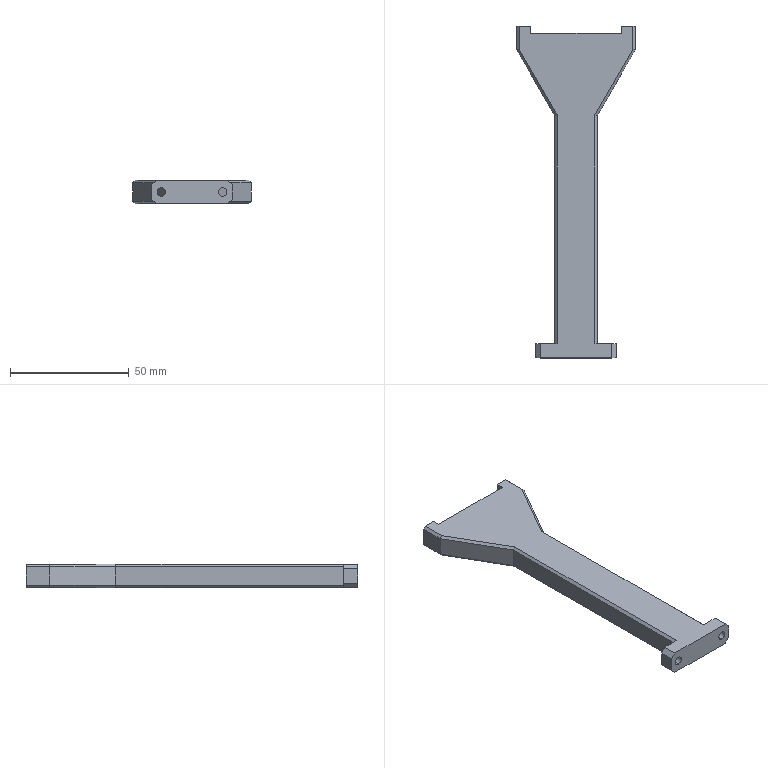Part | SolidWorks | features Chamfer 2, HoleWzd 2, ICE 2, Extrusion 1, MirrorPattern 1 | 1 solid | 46 faces | box 50 x 140 x 10 mm | volume 32128 mm3 | plane 34 | cylinder 8 | cone 4 | commonest cylinder face diameters 2.5 x4 3.5 x4
STEP:
#1=CARTESIAN_POINT('',(-13.,-64.,1.75));
#2=VERTEX_POINT('',#1);
#3=CARTESIAN_POINT('',(-13.,-64.,-1.75));
#4=VERTEX_POINT('',#3);
#5=CARTESIAN_POINT('',(-13.,-64.,0.));
#6=DIRECTION('',(0.,-1.,0.));
#7=DIRECTION('',(0.,0.,-1.));
#8=AXIS2_PLACEMENT_3D('',#5,#6,#7);
#9=CIRCLE('',#8,1.75);
#10=EDGE_CURVE('',#2,#4,#9,.T.);
#11=ORIENTED_EDGE('',*,*,#10,.F.);
#12=CARTESIAN_POINT('',(-13.,-70.,1.75));
#13=VERTEX_POINT('',#12);
#14=CARTESIAN_POINT('',(-13.,-70.,1.75));
#15=DIRECTION('',(0.,-1.,0.));
#16=VECTOR('',#15,1000.);
#17=LINE('',#14,#16);
#18=EDGE_CURVE('',#2,#13,#17,.T.);
#19=ORIENTED_EDGE('',*,*,#18,.T.);
#20=CARTESIAN_POINT('',(-13.,-70.,-1.75));
#21=VERTEX_POINT('',#20);
#22=CARTESIAN_POINT('',(-13.,-70.,0.));
#23=DIRECTION('',(0.,-1.,0.));
#24=DIRECTION('',(0.,0.,-1.));
#25=AXIS2_PLACEMENT_3D('',#22,#23,#24);
#26=CIRCLE('',#25,1.75);
#27=EDGE_CURVE('',#13,#21,#26,.T.);
#28=ORIENTED_EDGE('',*,*,#27,.T.);
#29=CARTESIAN_POINT('',(-13.,-70.,-1.75));
#30=DIRECTION('',(0.,-1.,0.));
#31=VECTOR('',#30,1000.);
#32=LINE('',#29,#31);
#33=EDGE_CURVE('',#4,#21,#32,.T.);
#34=ORIENTED_EDGE('',*,*,#33,.F.);
#35=EDGE_LOOP('',(#11,#19,#28,#34));
#36=FACE_OUTER_BOUND('',#35,.T.);
#37=CARTESIAN_POINT('',(-13.,-70.,0.));
#38=DIRECTION('',(0.,-1.,0.));
#39=DIRECTION('',(0.,0.,-1.));
#40=AXIS2_PLACEMENT_3D('',#37,#38,#39);
#41=CYLINDRICAL_SURFACE('',#40,1.75);
#42=ADVANCED_FACE('',(#36),#41,.F.);
#43=CARTESIAN_POINT('',(13.,-64.,-1.75));
#44=VERTEX_POINT('',#43);
#45=CARTESIAN_POINT('',(13.,-64.,1.75));
#46=VERTEX_POINT('',#45);
#47=CARTESIAN_POINT('',(13.,-64.,0.));
#48=DIRECTION('',(0.,1.,0.));
#49=DIRECTION('',(0.,0.,1.));
#50=AXIS2_PLACEMENT_3D('',#47,#48,#49);
#51=CIRCLE('',#50,1.75);
#52=EDGE_CURVE('',#44,#46,#51,.T.);
#53=ORIENTED_EDGE('',*,*,#52,.T.);
#54=CARTESIAN_POINT('',(13.,-70.,1.75));
#55=VERTEX_POINT('',#54);
#56=CARTESIAN_POINT('',(13.,-70.,1.75));
#57=DIRECTION('',(0.,-1.,0.));
#58=VECTOR('',#57,1000.);
#59=LINE('',#56,#58);
#60=EDGE_CURVE('',#46,#55,#59,.T.);
#61=ORIENTED_EDGE('',*,*,#60,.T.);
#62=CARTESIAN_POINT('',(13.,-70.,-1.75));
#63=VERTEX_POINT('',#62);
#64=CARTESIAN_POINT('',(13.,-70.,0.));
#65=DIRECTION('',(0.,-1.,0.));
#66=DIRECTION('',(0.,0.,-1.));
#67=AXIS2_PLACEMENT_3D('',#64,#65,#66);
#68=CIRCLE('',#67,1.75);
#69=EDGE_CURVE('',#55,#63,#68,.T.);
#70=ORIENTED_EDGE('',*,*,#69,.T.);
#71=CARTESIAN_POINT('',(13.,-70.,-1.75));
#72=DIRECTION('',(0.,-1.,0.));
#73=VECTOR('',#72,1000.);
#74=LINE('',#71,#73);
#75=EDGE_CURVE('',#44,#63,#74,.T.);
#76=ORIENTED_EDGE('',*,*,#75,.F.);
#77=EDGE_LOOP('',(#53,#61,#70,#76));
#78=FACE_OUTER_BOUND('',#77,.T.);
#79=CARTESIAN_POINT('',(13.,-70.,0.));
#80=DIRECTION('',(0.,-1.,0.));
#81=DIRECTION('',(0.,0.,-1.));
#82=AXIS2_PLACEMENT_3D('',#79,#80,#81);
#83=CYLINDRICAL_SURFACE('',#82,1.75);
#84=ADVANCED_FACE('',(#78),#83,.F.);
#85=CARTESIAN_POINT('',(-22.,61.5,-1.25));
#86=VERTEX_POINT('',#85);
#87=CARTESIAN_POINT('',(-22.,61.5,1.25));
#88=VERTEX_POINT('',#87);
#89=CARTESIAN_POINT('',(-22.,61.5,0.));
#90=DIRECTION('',(0.,1.,0.));
#91=DIRECTION('',(0.,0.,1.));
#92=AXIS2_PLACEMENT_3D('',#89,#90,#91);
#93=CIRCLE('',#92,1.25);
#94=EDGE_CURVE('',#86,#88,#93,.T.);
#95=ORIENTED_EDGE('',*,*,#94,.F.);
#96=CARTESIAN_POINT('',(-22.,70.,-1.25));
#97=VERTEX_POINT('',#96);
#98=CARTESIAN_POINT('',(-22.,70.,-1.25));
#99=DIRECTION('',(0.,1.,0.));
#100=VECTOR('',#99,1000.);
#101=LINE('',#98,#100);
#102=EDGE_CURVE('',#86,#97,#101,.T.);
#103=ORIENTED_EDGE('',*,*,#102,.T.);
#104=CARTESIAN_POINT('',(-22.,70.,1.25));
#105=VERTEX_POINT('',#104);
#106=CARTESIAN_POINT('',(-22.,70.,0.));
#107=DIRECTION('',(0.,1.,0.));
#108=DIRECTION('',(0.,0.,1.));
#109=AXIS2_PLACEMENT_3D('',#106,#107,#108);
#110=CIRCLE('',#109,1.25);
#111=EDGE_CURVE('',#97,#105,#110,.T.);
#112=ORIENTED_EDGE('',*,*,#111,.T.);
#113=CARTESIAN_POINT('',(-22.,70.,1.25));
#114=DIRECTION('',(0.,1.,0.));
#115=VECTOR('',#114,1000.);
#116=LINE('',#113,#115);
#117=EDGE_CURVE('',#88,#105,#116,.T.);
#118=ORIENTED_EDGE('',*,*,#117,.F.);
#119=EDGE_LOOP('',(#95,#103,#112,#118));
#120=FACE_OUTER_BOUND('',#119,.T.);
#121=CARTESIAN_POINT('',(-22.,70.,0.));
#122=DIRECTION('',(0.,1.,0.));
#123=DIRECTION('',(0.,0.,1.));
#124=AXIS2_PLACEMENT_3D('',#121,#122,#123);
#125=CYLINDRICAL_SURFACE('',#124,1.25);
#126=ADVANCED_FACE('',(#120),#125,.F.);
#127=CARTESIAN_POINT('',(-22.,60.749,0.));
#128=VERTEX_POINT('',#127);
#129=CARTESIAN_POINT('',(-22.,61.5,1.25));
#130=DIRECTION('',(0.,0.515,0.8572));
#131=VECTOR('',#130,1000.);
#132=LINE('',#129,#131);
#133=EDGE_CURVE('',#128,#88,#132,.T.);
#134=ORIENTED_EDGE('',*,*,#133,.F.);
#135=CARTESIAN_POINT('',(-22.,61.5,-1.25));
#136=DIRECTION('',(0.,0.515,-0.8572));
#137=VECTOR('',#136,1000.);
#138=LINE('',#135,#137);
#139=EDGE_CURVE('',#128,#86,#138,.T.);
#140=ORIENTED_EDGE('',*,*,#139,.T.);
#141=ORIENTED_EDGE('',*,*,#94,.T.);
#142=EDGE_LOOP('',(#134,#140,#141));
#143=FACE_OUTER_BOUND('',#142,.T.);
#144=CARTESIAN_POINT('',(-22.,61.5,0.));
#145=DIRECTION('',(0.,1.,0.));
#146=DIRECTION('',(0.,0.,1.));
#147=AXIS2_PLACEMENT_3D('',#144,#145,#146);
#148=CONICAL_SURFACE('',#147,1.25,1.03);
#149=ADVANCED_FACE('',(#143),#148,.F.);
#150=CARTESIAN_POINT('',(22.,61.5,-1.25));
#151=VERTEX_POINT('',#150);
#152=CARTESIAN_POINT('',(22.,61.5,1.25));
#153=VERTEX_POINT('',#152);
#154=CARTESIAN_POINT('',(22.,61.5,0.));
#155=DIRECTION('',(0.,1.,0.));
#156=DIRECTION('',(0.,0.,1.));
#157=AXIS2_PLACEMENT_3D('',#154,#155,#156);
#158=CIRCLE('',#157,1.25);
#159=EDGE_CURVE('',#151,#153,#158,.T.);
#160=ORIENTED_EDGE('',*,*,#159,.F.);
#161=CARTESIAN_POINT('',(22.,70.,-1.25));
#162=VERTEX_POINT('',#161);
#163=CARTESIAN_POINT('',(22.,70.,-1.25));
#164=DIRECTION('',(0.,1.,0.));
#165=VECTOR('',#164,1000.);
#166=LINE('',#163,#165);
#167=EDGE_CURVE('',#151,#162,#166,.T.);
#168=ORIENTED_EDGE('',*,*,#167,.T.);
#169=CARTESIAN_POINT('',(22.,70.,1.25));
#170=VERTEX_POINT('',#169);
#171=CARTESIAN_POINT('',(22.,70.,0.));
#172=DIRECTION('',(0.,1.,0.));
#173=DIRECTION('',(0.,0.,1.));
#174=AXIS2_PLACEMENT_3D('',#171,#172,#173);
#175=CIRCLE('',#174,1.25);
#176=EDGE_CURVE('',#162,#170,#175,.T.);
#177=ORIENTED_EDGE('',*,*,#176,.T.);
#178=CARTESIAN_POINT('',(22.,70.,1.25));
#179=DIRECTION('',(0.,1.,0.));
#180=VECTOR('',#179,1000.);
#181=LINE('',#178,#180);
#182=EDGE_CURVE('',#153,#170,#181,.T.);
#183=ORIENTED_EDGE('',*,*,#182,.F.);
#184=EDGE_LOOP('',(#160,#168,#177,#183));
#185=FACE_OUTER_BOUND('',#184,.T.);
#186=CARTESIAN_POINT('',(22.,70.,0.));
#187=DIRECTION('',(0.,1.,0.));
#188=DIRECTION('',(0.,0.,1.));
#189=AXIS2_PLACEMENT_3D('',#186,#187,#188);
#190=CYLINDRICAL_SURFACE('',#189,1.25);
#191=ADVANCED_FACE('',(#185),#190,.F.);
#192=CARTESIAN_POINT('',(22.,60.749,0.));
#193=VERTEX_POINT('',#192);
#194=CARTESIAN_POINT('',(22.,61.5,1.25));
#195=DIRECTION('',(0.,0.515,0.8572));
#196=VECTOR('',#195,1000.);
#197=LINE('',#194,#196);
#198=EDGE_CURVE('',#193,#153,#197,.T.);
#199=ORIENTED_EDGE('',*,*,#198,.F.);
#200=CARTESIAN_POINT('',(22.,61.5,-1.25));
#201=DIRECTION('',(0.,0.515,-0.8572));
#202=VECTOR('',#201,1000.);
#203=LINE('',#200,#202);
#204=EDGE_CURVE('',#193,#151,#203,.T.);
#205=ORIENTED_EDGE('',*,*,#204,.T.);
#206=ORIENTED_EDGE('',*,*,#159,.T.);
#207=EDGE_LOOP('',(#199,#205,#206));
#208=FACE_OUTER_BOUND('',#207,.T.);
#209=CARTESIAN_POINT('',(22.,61.5,0.));
#210=DIRECTION('',(0.,1.,0.));
#211=DIRECTION('',(0.,0.,1.));
#212=AXIS2_PLACEMENT_3D('',#209,#210,#211);
#213=CONICAL_SURFACE('',#212,1.25,1.03);
#214=ADVANCED_FACE('',(#208),#213,.F.);
#215=CARTESIAN_POINT('',(22.,70.,0.));
#216=DIRECTION('',(0.,1.,0.));
#217=DIRECTION('',(0.,0.,1.));
#218=AXIS2_PLACEMENT_3D('',#215,#216,#217);
#219=CIRCLE('',#218,1.25);
#220=EDGE_CURVE('',#170,#162,#219,.T.);
#221=ORIENTED_EDGE('',*,*,#220,.F.);
#222=ORIENTED_EDGE('',*,*,#176,.F.);
#223=EDGE_LOOP('',(#221,#222));
#224=FACE_BOUND('',#223,.T.);
#225=CARTESIAN_POINT('',(25.,70.,4.));
#226=VERTEX_POINT('',#225);
#227=CARTESIAN_POINT('',(25.,70.,-4.));
#228=VERTEX_POINT('',#227);
#229=CARTESIAN_POINT('',(25.,70.,5.));
#230=DIRECTION('',(0.,0.,-1.));
#231=VECTOR('',#230,1000.);
#232=LINE('',#229,#231);
#233=EDGE_CURVE('',#226,#228,#232,.T.);
#234=ORIENTED_EDGE('',*,*,#233,.T.);
#235=CARTESIAN_POINT('',(24.,70.,-5.));
#236=VERTEX_POINT('',#235);
#237=CARTESIAN_POINT('',(25.,70.,-4.));
#238=DIRECTION('',(-0.7071,0.,-0.7071));
#239=VECTOR('',#238,1000.);
#240=LINE('',#237,#239);
#241=EDGE_CURVE('',#228,#236,#240,.T.);
#242=ORIENTED_EDGE('',*,*,#241,.T.);
#243=CARTESIAN_POINT('',(19.,70.,-5.));
#244=VERTEX_POINT('',#243);
#245=CARTESIAN_POINT('',(-25.,70.,-5.));
#246=DIRECTION('',(-1.,0.,0.));
#247=VECTOR('',#246,1000.);
#248=LINE('',#245,#247);
#249=EDGE_CURVE('',#236,#244,#248,.T.);
#250=ORIENTED_EDGE('',*,*,#249,.T.);
#251=CARTESIAN_POINT('',(19.,70.,5.));
#252=VERTEX_POINT('',#251);
#253=CARTESIAN_POINT('',(19.,70.,-5.));
#254=DIRECTION('',(0.,0.,1.));
#255=VECTOR('',#254,1000.);
#256=LINE('',#253,#255);
#257=EDGE_CURVE('',#244,#252,#256,.T.);
#258=ORIENTED_EDGE('',*,*,#257,.T.);
#259=CARTESIAN_POINT('',(24.,70.,5.));
#260=VERTEX_POINT('',#259);
#261=CARTESIAN_POINT('',(-25.,70.,5.));
#262=DIRECTION('',(-1.,0.,0.));
#263=VECTOR('',#262,1000.);
#264=LINE('',#261,#263);
#265=EDGE_CURVE('',#260,#252,#264,.T.);
#266=ORIENTED_EDGE('',*,*,#265,.F.);
#267=CARTESIAN_POINT('',(24.,70.,5.));
#268=DIRECTION('',(0.7071,0.,-0.7071));
#269=VECTOR('',#268,1000.);
#270=LINE('',#267,#269);
#271=EDGE_CURVE('',#260,#226,#270,.T.);
#272=ORIENTED_EDGE('',*,*,#271,.T.);
#273=EDGE_LOOP('',(#234,#242,#250,#258,#266,#272));
#274=FACE_OUTER_BOUND('',#273,.T.);
#275=CARTESIAN_POINT('',(-25.,70.,5.));
#276=DIRECTION('',(0.,-1.,0.));
#277=DIRECTION('',(0.,0.,-1.));
#278=AXIS2_PLACEMENT_3D('',#275,#276,#277);
#279=PLANE('',#278);
#280=ADVANCED_FACE('',(#224,#274),#279,.F.);
#281=CARTESIAN_POINT('',(25.,60.,-4.));
#282=VERTEX_POINT('',#281);
#283=CARTESIAN_POINT('',(25.,60.,4.));
#284=VERTEX_POINT('',#283);
#285=CARTESIAN_POINT('',(25.,60.,-5.));
#286=DIRECTION('',(0.,0.,1.));
#287=VECTOR('',#286,1000.);
#288=LINE('',#285,#287);
#289=EDGE_CURVE('',#282,#284,#288,.T.);
#290=ORIENTED_EDGE('',*,*,#289,.F.);
#291=CARTESIAN_POINT('',(25.,70.,-4.));
#292=DIRECTION('',(0.,1.,0.));
#293=VECTOR('',#292,1000.);
#294=LINE('',#291,#293);
#295=EDGE_CURVE('',#282,#228,#294,.T.);
#296=ORIENTED_EDGE('',*,*,#295,.T.);
#297=ORIENTED_EDGE('',*,*,#233,.F.);
#298=CARTESIAN_POINT('',(25.,60.,4.));
#299=DIRECTION('',(0.,-1.,0.));
#300=VECTOR('',#299,1000.);
#301=LINE('',#298,#300);
#302=EDGE_CURVE('',#226,#284,#301,.T.);
#303=ORIENTED_EDGE('',*,*,#302,.T.);
#304=EDGE_LOOP('',(#290,#296,#297,#303));
#305=FACE_OUTER_BOUND('',#304,.T.);
#306=CARTESIAN_POINT('',(25.,70.,5.));
#307=DIRECTION('',(-1.,0.,0.));
#308=DIRECTION('',(0.,-1.,0.));
#309=AXIS2_PLACEMENT_3D('',#306,#307,#308);
#310=PLANE('',#309);
#311=ADVANCED_FACE('',(#305),#310,.F.);
#312=CARTESIAN_POINT('',(-13.,-70.,0.));
#313=DIRECTION('',(0.,-1.,0.));
#314=DIRECTION('',(0.,0.,-1.));
#315=AXIS2_PLACEMENT_3D('',#312,#313,#314);
#316=CIRCLE('',#315,1.75);
#317=EDGE_CURVE('',#21,#13,#316,.T.);
#318=ORIENTED_EDGE('',*,*,#317,.F.);
#319=ORIENTED_EDGE('',*,*,#27,.F.);
#320=EDGE_LOOP('',(#318,#319));
#321=FACE_BOUND('',#320,.T.);
#322=CARTESIAN_POINT('',(13.,-70.,0.));
#323=DIRECTION('',(0.,-1.,0.));
#324=DIRECTION('',(0.,0.,-1.));
#325=AXIS2_PLACEMENT_3D('',#322,#323,#324);
#326=CIRCLE('',#325,1.75);
#327=EDGE_CURVE('',#63,#55,#326,.T.);
#328=ORIENTED_EDGE('',*,*,#327,.F.);
#329=ORIENTED_EDGE('',*,*,#69,.F.);
#330=EDGE_LOOP('',(#328,#329));
#331=FACE_BOUND('',#330,.T.);
#332=CARTESIAN_POINT('',(-17.,-70.,-3.));
#333=VERTEX_POINT('',#332);
#334=CARTESIAN_POINT('',(-17.,-70.,3.));
#335=VERTEX_POINT('',#334);
#336=CARTESIAN_POINT('',(-17.,-70.,-5.));
#337=DIRECTION('',(0.,0.,1.));
#338=VECTOR('',#337,1000.);
#339=LINE('',#336,#338);
#340=EDGE_CURVE('',#333,#335,#339,.T.);
#341=ORIENTED_EDGE('',*,*,#340,.F.);
#342=CARTESIAN_POINT('',(-15.,-70.,-5.));
#343=VERTEX_POINT('',#342);
#344=CARTESIAN_POINT('',(-15.,-70.,-5.));
#345=DIRECTION('',(0.7071,0.,-0.7071));
#346=VECTOR('',#345,1000.);
#347=LINE('',#344,#346);
#348=EDGE_CURVE('',#333,#343,#347,.T.);
#349=ORIENTED_EDGE('',*,*,#348,.T.);
#350=CARTESIAN_POINT('',(15.,-70.,-5.));
#351=VERTEX_POINT('',#350);
#352=CARTESIAN_POINT('',(-25.,-70.,-5.));
#353=DIRECTION('',(1.,0.,0.));
#354=VECTOR('',#353,1000.);
#355=LINE('',#352,#354);
#356=EDGE_CURVE('',#343,#351,#355,.T.);
#357=ORIENTED_EDGE('',*,*,#356,.T.);
#358=CARTESIAN_POINT('',(17.,-70.,-3.));
#359=VERTEX_POINT('',#358);
#360=CARTESIAN_POINT('',(17.,-70.,-3.));
#361=DIRECTION('',(0.7071,0.,0.7071));
#362=VECTOR('',#361,1000.);
#363=LINE('',#360,#362);
#364=EDGE_CURVE('',#351,#359,#363,.T.);
#365=ORIENTED_EDGE('',*,*,#364,.T.);
#366=CARTESIAN_POINT('',(17.,-70.,3.));
#367=VERTEX_POINT('',#366);
#368=CARTESIAN_POINT('',(17.,-70.,-5.));
#369=DIRECTION('',(0.,0.,1.));
#370=VECTOR('',#369,1000.);
#371=LINE('',#368,#370);
#372=EDGE_CURVE('',#359,#367,#371,.T.);
#373=ORIENTED_EDGE('',*,*,#372,.T.);
#374=CARTESIAN_POINT('',(15.,-70.,5.));
#375=VERTEX_POINT('',#374);
#376=CARTESIAN_POINT('',(15.,-70.,5.));
#377=DIRECTION('',(-0.7071,0.,0.7071));
#378=VECTOR('',#377,1000.);
#379=LINE('',#376,#378);
#380=EDGE_CURVE('',#367,#375,#379,.T.);
#381=ORIENTED_EDGE('',*,*,#380,.T.);
#382=CARTESIAN_POINT('',(-15.,-70.,5.));
#383=VERTEX_POINT('',#382);
#384=CARTESIAN_POINT('',(-25.,-70.,5.));
#385=DIRECTION('',(1.,0.,0.));
#386=VECTOR('',#385,1000.);
#387=LINE('',#384,#386);
#388=EDGE_CURVE('',#383,#375,#387,.T.);
#389=ORIENTED_EDGE('',*,*,#388,.F.);
#390=CARTESIAN_POINT('',(-17.,-70.,3.));
#391=DIRECTION('',(-0.7071,0.,-0.7071));
#392=VECTOR('',#391,1000.);
#393=LINE('',#390,#392);
#394=EDGE_CURVE('',#383,#335,#393,.T.);
#395=ORIENTED_EDGE('',*,*,#394,.T.);
#396=EDGE_LOOP('',(#341,#349,#357,#365,#373,#381,#389,#395));
#397=FACE_OUTER_BOUND('',#396,.T.);
#398=CARTESIAN_POINT('',(-25.,-70.,5.));
#399=DIRECTION('',(0.,1.,0.));
#400=DIRECTION('',(0.,0.,1.));
#401=AXIS2_PLACEMENT_3D('',#398,#399,#400);
#402=PLANE('',#401);
#403=ADVANCED_FACE('',(#321,#331,#397),#402,.F.);
#404=CARTESIAN_POINT('',(-19.,70.,5.));
#405=VERTEX_POINT('',#404);
#406=CARTESIAN_POINT('',(-24.,70.,5.));
#407=VERTEX_POINT('',#406);
#408=CARTESIAN_POINT('',(-25.,70.,5.));
#409=DIRECTION('',(-1.,0.,0.));
#410=VECTOR('',#409,1000.);
#411=LINE('',#408,#410);
#412=EDGE_CURVE('',#405,#407,#411,.T.);
#413=ORIENTED_EDGE('',*,*,#412,.T.);
#414=CARTESIAN_POINT('',(-24.,60.268,5.));
#415=VERTEX_POINT('',#414);
#416=CARTESIAN_POINT('',(-24.,60.,5.));
#417=DIRECTION('',(0.,-1.,0.));
#418=VECTOR('',#417,1000.);
#419=LINE('',#416,#418);
#420=EDGE_CURVE('',#407,#415,#419,.T.);
#421=ORIENTED_EDGE('',*,*,#420,.T.);
#422=CARTESIAN_POINT('',(-8.,32.555,5.));
#423=VERTEX_POINT('',#422);
#424=CARTESIAN_POINT('',(-8.134,32.787,5.));
#425=DIRECTION('',(0.5,-0.866,0.));
#426=VECTOR('',#425,1000.);
#427=LINE('',#424,#426);
#428=EDGE_CURVE('',#415,#423,#427,.T.);
#429=ORIENTED_EDGE('',*,*,#428,.T.);
#430=CARTESIAN_POINT('',(-8.,-64.,5.));
#431=VERTEX_POINT('',#430);
#432=CARTESIAN_POINT('',(-8.,-64.,5.));
#433=DIRECTION('',(0.,-1.,0.));
#434=VECTOR('',#433,1000.);
#435=LINE('',#432,#434);
#436=EDGE_CURVE('',#423,#431,#435,.T.);
#437=ORIENTED_EDGE('',*,*,#436,.T.);
#438=CARTESIAN_POINT('',(-15.,-64.,5.));
#439=VERTEX_POINT('',#438);
#440=CARTESIAN_POINT('',(-9.,-64.,5.));
#441=DIRECTION('',(1.,0.,0.));
#442=VECTOR('',#441,1000.);
#443=LINE('',#440,#442);
#444=EDGE_CURVE('',#439,#431,#443,.T.);
#445=ORIENTED_EDGE('',*,*,#444,.F.);
#446=CARTESIAN_POINT('',(-15.,-70.,5.));
#447=DIRECTION('',(0.,-1.,0.));
#448=VECTOR('',#447,1000.);
#449=LINE('',#446,#448);
#450=EDGE_CURVE('',#439,#383,#449,.T.);
#451=ORIENTED_EDGE('',*,*,#450,.T.);
#452=ORIENTED_EDGE('',*,*,#388,.T.);
#453=CARTESIAN_POINT('',(15.,-64.,5.));
#454=VERTEX_POINT('',#453);
#455=CARTESIAN_POINT('',(15.,0.,5.));
#456=DIRECTION('',(0.,1.,0.));
#457=VECTOR('',#456,1000.);
#458=LINE('',#455,#457);
#459=EDGE_CURVE('',#375,#454,#458,.T.);
#460=ORIENTED_EDGE('',*,*,#459,.T.);
#461=CARTESIAN_POINT('',(8.,-64.,5.));
#462=VERTEX_POINT('',#461);
#463=CARTESIAN_POINT('',(9.,-64.,5.));
#464=DIRECTION('',(-1.,0.,0.));
#465=VECTOR('',#464,1000.);
#466=LINE('',#463,#465);
#467=EDGE_CURVE('',#454,#462,#466,.T.);
#468=ORIENTED_EDGE('',*,*,#467,.T.);
#469=CARTESIAN_POINT('',(8.,32.555,5.));
#470=VERTEX_POINT('',#469);
#471=CARTESIAN_POINT('',(8.,0.,5.));
#472=DIRECTION('',(0.,1.,0.));
#473=VECTOR('',#472,1000.);
#474=LINE('',#471,#473);
#475=EDGE_CURVE('',#462,#470,#474,.T.);
#476=ORIENTED_EDGE('',*,*,#475,.T.);
#477=CARTESIAN_POINT('',(24.,60.268,5.));
#478=VERTEX_POINT('',#477);
#479=CARTESIAN_POINT('',(-8.097,4.675,5.));
#480=DIRECTION('',(0.5,0.866,0.));
#481=VECTOR('',#480,1000.);
#482=LINE('',#479,#481);
#483=EDGE_CURVE('',#470,#478,#482,.T.);
#484=ORIENTED_EDGE('',*,*,#483,.T.);
#485=CARTESIAN_POINT('',(24.,70.,5.));
#486=DIRECTION('',(0.,1.,0.));
#487=VECTOR('',#486,1000.);
#488=LINE('',#485,#487);
#489=EDGE_CURVE('',#478,#260,#488,.T.);
#490=ORIENTED_EDGE('',*,*,#489,.T.);
#491=ORIENTED_EDGE('',*,*,#265,.T.);
#492=CARTESIAN_POINT('',(19.,67.,5.));
#493=VERTEX_POINT('',#492);
#494=CARTESIAN_POINT('',(19.,70.,5.));
#495=DIRECTION('',(0.,1.,0.));
#496=VECTOR('',#495,1000.);
#497=LINE('',#494,#496);
#498=EDGE_CURVE('',#493,#252,#497,.T.);
#499=ORIENTED_EDGE('',*,*,#498,.F.);
#500=CARTESIAN_POINT('',(-19.,67.,5.));
#501=VERTEX_POINT('',#500);
#502=CARTESIAN_POINT('',(-19.,67.,5.));
#503=DIRECTION('',(1.,0.,0.));
#504=VECTOR('',#503,1000.);
#505=LINE('',#502,#504);
#506=EDGE_CURVE('',#501,#493,#505,.T.);
#507=ORIENTED_EDGE('',*,*,#506,.F.);
#508=CARTESIAN_POINT('',(-19.,70.,5.));
#509=DIRECTION('',(0.,-1.,0.));
#510=VECTOR('',#509,1000.);
#511=LINE('',#508,#510);
#512=EDGE_CURVE('',#405,#501,#511,.T.);
#513=ORIENTED_EDGE('',*,*,#512,.F.);
#514=EDGE_LOOP('',(#413,#421,#429,#437,#445,#451,#452,#460,#468,#476,#484,#490,#491,#499,#507,#513));
#515=FACE_OUTER_BOUND('',#514,.T.);
#516=CARTESIAN_POINT('',(0.,0.,5.));
#517=DIRECTION('',(0.,0.,1.));
#518=DIRECTION('',(1.,0.,0.));
#519=AXIS2_PLACEMENT_3D('',#516,#517,#518);
#520=PLANE('',#519);
#521=ADVANCED_FACE('',(#515),#520,.T.);
#522=CARTESIAN_POINT('',(-8.,32.555,-5.));
#523=VERTEX_POINT('',#522);
#524=CARTESIAN_POINT('',(-24.,60.268,-5.));
#525=VERTEX_POINT('',#524);
#526=CARTESIAN_POINT('',(8.097,4.675,-5.));
#527=DIRECTION('',(-0.5,0.866,0.));
#528=VECTOR('',#527,1000.);
#529=LINE('',#526,#528);
#530=EDGE_CURVE('',#523,#525,#529,.T.);
#531=ORIENTED_EDGE('',*,*,#530,.T.);
#532=CARTESIAN_POINT('',(-24.,70.,-5.));
#533=VERTEX_POINT('',#532);
#534=CARTESIAN_POINT('',(-24.,0.,-5.));
#535=DIRECTION('',(0.,1.,0.));
#536=VECTOR('',#535,1000.);
#537=LINE('',#534,#536);
#538=EDGE_CURVE('',#525,#533,#537,.T.);
#539=ORIENTED_EDGE('',*,*,#538,.T.);
#540=CARTESIAN_POINT('',(-19.,70.,-5.));
#541=VERTEX_POINT('',#540);
#542=CARTESIAN_POINT('',(-25.,70.,-5.));
#543=DIRECTION('',(-1.,0.,0.));
#544=VECTOR('',#543,1000.);
#545=LINE('',#542,#544);
#546=EDGE_CURVE('',#541,#533,#545,.T.);
#547=ORIENTED_EDGE('',*,*,#546,.F.);
#548=CARTESIAN_POINT('',(-19.,67.,-5.));
#549=VERTEX_POINT('',#548);
#550=CARTESIAN_POINT('',(-19.,70.,-5.));
#551=DIRECTION('',(0.,-1.,0.));
#552=VECTOR('',#551,1000.);
#553=LINE('',#550,#552);
#554=EDGE_CURVE('',#541,#549,#553,.T.);
#555=ORIENTED_EDGE('',*,*,#554,.T.);
#556=CARTESIAN_POINT('',(19.,67.,-5.));
#557=VERTEX_POINT('',#556);
#558=CARTESIAN_POINT('',(-19.,67.,-5.));
#559=DIRECTION('',(1.,0.,0.));
#560=VECTOR('',#559,1000.);
#561=LINE('',#558,#560);
#562=EDGE_CURVE('',#549,#557,#561,.T.);
#563=ORIENTED_EDGE('',*,*,#562,.T.);
#564=CARTESIAN_POINT('',(19.,70.,-5.));
#565=DIRECTION('',(0.,1.,0.));
#566=VECTOR('',#565,1000.);
#567=LINE('',#564,#566);
#568=EDGE_CURVE('',#557,#244,#567,.T.);
#569=ORIENTED_EDGE('',*,*,#568,.T.);
#570=ORIENTED_EDGE('',*,*,#249,.F.);
#571=CARTESIAN_POINT('',(24.,60.268,-5.));
#572=VERTEX_POINT('',#571);
#573=CARTESIAN_POINT('',(24.,0.,-5.));
#574=DIRECTION('',(0.,-1.,0.));
#575=VECTOR('',#574,1000.);
#576=LINE('',#573,#575);
#577=EDGE_CURVE('',#236,#572,#576,.T.);
#578=ORIENTED_EDGE('',*,*,#577,.T.);
#579=CARTESIAN_POINT('',(8.,32.555,-5.));
#580=VERTEX_POINT('',#579);
#581=CARTESIAN_POINT('',(8.134,32.787,-5.));
#582=DIRECTION('',(-0.5,-0.866,0.));
#583=VECTOR('',#582,1000.);
#584=LINE('',#581,#583);
#585=EDGE_CURVE('',#572,#580,#584,.T.);
#586=ORIENTED_EDGE('',*,*,#585,.T.);
#587=CARTESIAN_POINT('',(8.,-64.,-5.));
#588=VERTEX_POINT('',#587);
#589=CARTESIAN_POINT('',(8.,-64.,-5.));
#590=DIRECTION('',(0.,-1.,0.));
#591=VECTOR('',#590,1000.);
#592=LINE('',#589,#591);
#593=EDGE_CURVE('',#580,#588,#592,.T.);
#594=ORIENTED_EDGE('',*,*,#593,.T.);
#595=CARTESIAN_POINT('',(15.,-64.,-5.));
#596=VERTEX_POINT('',#595);
#597=CARTESIAN_POINT('',(9.,-64.,-5.));
#598=DIRECTION('',(-1.,0.,0.));
#599=VECTOR('',#598,1000.);
#600=LINE('',#597,#599);
#601=EDGE_CURVE('',#596,#588,#600,.T.);
#602=ORIENTED_EDGE('',*,*,#601,.F.);
#603=CARTESIAN_POINT('',(15.,-70.,-5.));
#604=DIRECTION('',(0.,-1.,0.));
#605=VECTOR('',#604,1000.);
#606=LINE('',#603,#605);
#607=EDGE_CURVE('',#596,#351,#606,.T.);
#608=ORIENTED_EDGE('',*,*,#607,.T.);
#609=ORIENTED_EDGE('',*,*,#356,.F.);
#610=CARTESIAN_POINT('',(-15.,-64.,-5.));
#611=VERTEX_POINT('',#610);
#612=CARTESIAN_POINT('',(-15.,0.,-5.));
#613=DIRECTION('',(0.,1.,0.));
#614=VECTOR('',#613,1000.);
#615=LINE('',#612,#614);
#616=EDGE_CURVE('',#343,#611,#615,.T.);
#617=ORIENTED_EDGE('',*,*,#616,.T.);
#618=CARTESIAN_POINT('',(-8.,-64.,-5.));
#619=VERTEX_POINT('',#618);
#620=CARTESIAN_POINT('',(-9.,-64.,-5.));
#621=DIRECTION('',(1.,0.,0.));
#622=VECTOR('',#621,1000.);
#623=LINE('',#620,#622);
#624=EDGE_CURVE('',#611,#619,#623,.T.);
#625=ORIENTED_EDGE('',*,*,#624,.T.);
#626=CARTESIAN_POINT('',(-8.,0.,-5.));
#627=DIRECTION('',(0.,1.,0.));
#628=VECTOR('',#627,1000.);
#629=LINE('',#626,#628);
#630=EDGE_CURVE('',#619,#523,#629,.T.);
#631=ORIENTED_EDGE('',*,*,#630,.T.);
#632=EDGE_LOOP('',(#531,#539,#547,#555,#563,#569,#570,#578,#586,#594,#602,#608,#609,#617,#625,#631));
#633=FACE_OUTER_BOUND('',#632,.T.);
#634=CARTESIAN_POINT('',(0.,0.,-5.));
#635=DIRECTION('',(0.,0.,1.));
#636=DIRECTION('',(1.,0.,0.));
#637=AXIS2_PLACEMENT_3D('',#634,#635,#636);
#638=PLANE('',#637);
#639=ADVANCED_FACE('',(#633),#638,.F.);
#640=CARTESIAN_POINT('',(-22.,70.,0.));
#641=DIRECTION('',(0.,1.,0.));
#642=DIRECTION('',(0.,0.,1.));
#643=AXIS2_PLACEMENT_3D('',#640,#641,#642);
#644=CIRCLE('',#643,1.25);
#645=EDGE_CURVE('',#105,#97,#644,.T.);
#646=ORIENTED_EDGE('',*,*,#645,.F.);
#647=ORIENTED_EDGE('',*,*,#111,.F.);
#648=EDGE_LOOP('',(#646,#647));
#649=FACE_BOUND('',#648,.T.);
#650=ORIENTED_EDGE('',*,*,#546,.T.);
#651=CARTESIAN_POINT('',(-25.,70.,-4.));
#652=VERTEX_POINT('',#651);
#653=CARTESIAN_POINT('',(-25.,70.,-4.));
#654=DIRECTION('',(-0.7071,0.,0.7071));
#655=VECTOR('',#654,1000.);
#656=LINE('',#653,#655);
#657=EDGE_CURVE('',#533,#652,#656,.T.);
#658=ORIENTED_EDGE('',*,*,#657,.T.);
#659=CARTESIAN_POINT('',(-25.,70.,4.));
#660=VERTEX_POINT('',#659);
#661=CARTESIAN_POINT('',(-25.,70.,5.));
#662=DIRECTION('',(0.,0.,-1.));
#663=VECTOR('',#662,1000.);
#664=LINE('',#661,#663);
#665=EDGE_CURVE('',#660,#652,#664,.T.);
#666=ORIENTED_EDGE('',*,*,#665,.F.);
#667=CARTESIAN_POINT('',(-24.,70.,5.));
#668=DIRECTION('',(0.7071,0.,0.7071));
#669=VECTOR('',#668,1000.);
#670=LINE('',#667,#669);
#671=EDGE_CURVE('',#660,#407,#670,.T.);
#672=ORIENTED_EDGE('',*,*,#671,.T.);
#673=ORIENTED_EDGE('',*,*,#412,.F.);
#674=CARTESIAN_POINT('',(-19.,70.,-5.));
#675=DIRECTION('',(0.,0.,1.));
#676=VECTOR('',#675,1000.);
#677=LINE('',#674,#676);
#678=EDGE_CURVE('',#541,#405,#677,.T.);
#679=ORIENTED_EDGE('',*,*,#678,.F.);
#680=EDGE_LOOP('',(#650,#658,#666,#672,#673,#679));
#681=FACE_OUTER_BOUND('',#680,.T.);
#682=CARTESIAN_POINT('',(-25.,70.,5.));
#683=DIRECTION('',(0.,-1.,0.));
#684=DIRECTION('',(0.,0.,-1.));
#685=AXIS2_PLACEMENT_3D('',#682,#683,#684);
#686=PLANE('',#685);
#687=ADVANCED_FACE('',(#649,#681),#686,.F.);
#688=ORIENTED_EDGE('',*,*,#665,.T.);
#689=CARTESIAN_POINT('',(-25.,60.,-4.));
#690=VERTEX_POINT('',#689);
#691=CARTESIAN_POINT('',(-25.,70.,-4.));
#692=DIRECTION('',(0.,-1.,0.));
#693=VECTOR('',#692,1000.);
#694=LINE('',#691,#693);
#695=EDGE_CURVE('',#652,#690,#694,.T.);
#696=ORIENTED_EDGE('',*,*,#695,.T.);
#697=CARTESIAN_POINT('',(-25.,60.,4.));
#698=VERTEX_POINT('',#697);
#699=CARTESIAN_POINT('',(-25.,60.,-5.));
#700=DIRECTION('',(0.,0.,1.));
#701=VECTOR('',#700,1000.);
#702=LINE('',#699,#701);
#703=EDGE_CURVE('',#690,#698,#702,.T.);
#704=ORIENTED_EDGE('',*,*,#703,.T.);
#705=CARTESIAN_POINT('',(-25.,70.,4.));
#706=DIRECTION('',(0.,1.,0.));
#707=VECTOR('',#706,1000.);
#708=LINE('',#705,#707);
#709=EDGE_CURVE('',#698,#660,#708,.T.);
#710=ORIENTED_EDGE('',*,*,#709,.T.);
#711=EDGE_LOOP('',(#688,#696,#704,#710));
#712=FACE_OUTER_BOUND('',#711,.T.);
#713=CARTESIAN_POINT('',(-25.,70.,5.));
#714=DIRECTION('',(1.,0.,0.));
#715=DIRECTION('',(0.,1.,0.));
#716=AXIS2_PLACEMENT_3D('',#713,#714,#715);
#717=PLANE('',#716);
#718=ADVANCED_FACE('',(#712),#717,.F.);
#719=ORIENTED_EDGE('',*,*,#703,.F.);
#720=CARTESIAN_POINT('',(-9.,32.287,-4.));
#721=VERTEX_POINT('',#720);
#722=CARTESIAN_POINT('',(-25.,60.,-4.));
#723=DIRECTION('',(0.5,-0.866,0.));
#724=VECTOR('',#723,1000.);
#725=LINE('',#722,#724);
#726=EDGE_CURVE('',#690,#721,#725,.T.);
#727=ORIENTED_EDGE('',*,*,#726,.T.);
#728=CARTESIAN_POINT('',(-9.,32.287,4.));
#729=VERTEX_POINT('',#728);
#730=CARTESIAN_POINT('',(-9.,32.287,-5.));
#731=DIRECTION('',(0.,0.,1.));
#732=VECTOR('',#731,1000.);
#733=LINE('',#730,#732);
#734=EDGE_CURVE('',#721,#729,#733,.T.);
#735=ORIENTED_EDGE('',*,*,#734,.T.);
#736=CARTESIAN_POINT('',(-25.,60.,4.));
#737=DIRECTION('',(-0.5,0.866,0.));
#738=VECTOR('',#737,1000.);
#739=LINE('',#736,#738);
#740=EDGE_CURVE('',#729,#698,#739,.T.);
#741=ORIENTED_EDGE('',*,*,#740,.T.);
#742=EDGE_LOOP('',(#719,#727,#735,#741));
#743=FACE_OUTER_BOUND('',#742,.T.);
#744=CARTESIAN_POINT('',(-25.,60.,-5.));
#745=DIRECTION('',(0.866,0.5,0.));
#746=DIRECTION('',(-0.5,0.866,0.));
#747=AXIS2_PLACEMENT_3D('',#744,#745,#746);
#748=PLANE('',#747);
#749=ADVANCED_FACE('',(#743),#748,.F.);
#750=ORIENTED_EDGE('',*,*,#734,.F.);
#751=CARTESIAN_POINT('',(-9.,-64.,-4.));
#752=VERTEX_POINT('',#751);
#753=CARTESIAN_POINT('',(-9.,32.287,-4.));
#754=DIRECTION('',(0.,-1.,0.));
#755=VECTOR('',#754,1000.);
#756=LINE('',#753,#755);
#757=EDGE_CURVE('',#721,#752,#756,.T.);
#758=ORIENTED_EDGE('',*,*,#757,.T.);
#759=CARTESIAN_POINT('',(-9.,-64.,4.));
#760=VERTEX_POINT('',#759);
#761=CARTESIAN_POINT('',(-9.,-64.,-5.));
#762=DIRECTION('',(0.,0.,1.));
#763=VECTOR('',#762,1000.);
#764=LINE('',#761,#763);
#765=EDGE_CURVE('',#752,#760,#764,.T.);
#766=ORIENTED_EDGE('',*,*,#765,.T.);
#767=CARTESIAN_POINT('',(-9.,32.287,4.));
#768=DIRECTION('',(0.,1.,0.));
#769=VECTOR('',#768,1000.);
#770=LINE('',#767,#769);
#771=EDGE_CURVE('',#760,#729,#770,.T.);
#772=ORIENTED_EDGE('',*,*,#771,.T.);
#773=EDGE_LOOP('',(#750,#758,#766,#772));
#774=FACE_OUTER_BOUND('',#773,.T.);
#775=CARTESIAN_POINT('',(-9.,32.287,-5.));
#776=DIRECTION('',(1.,0.,0.));
#777=DIRECTION('',(0.,1.,0.));
#778=AXIS2_PLACEMENT_3D('',#775,#776,#777);
#779=PLANE('',#778);
#780=ADVANCED_FACE('',(#774),#779,.F.);
#781=CARTESIAN_POINT('',(-13.,-64.,0.));
#782=DIRECTION('',(0.,-1.,0.));
#783=DIRECTION('',(0.,0.,-1.));
#784=AXIS2_PLACEMENT_3D('',#781,#782,#783);
#785=CIRCLE('',#784,1.75);
#786=EDGE_CURVE('',#4,#2,#785,.T.);
#787=ORIENTED_EDGE('',*,*,#786,.T.);
#788=ORIENTED_EDGE('',*,*,#10,.T.);
#789=EDGE_LOOP('',(#787,#788));
#790=FACE_BOUND('',#789,.T.);
#791=ORIENTED_EDGE('',*,*,#624,.F.);
#792=CARTESIAN_POINT('',(-17.,-64.,-3.));
#793=VERTEX_POINT('',#792);
#794=CARTESIAN_POINT('',(-15.,-64.,-5.));
#795=DIRECTION('',(-0.7071,0.,0.7071));
#796=VECTOR('',#795,1000.);
#797=LINE('',#794,#796);
#798=EDGE_CURVE('',#611,#793,#797,.T.);
#799=ORIENTED_EDGE('',*,*,#798,.T.);
#800=CARTESIAN_POINT('',(-17.,-64.,3.));
#801=VERTEX_POINT('',#800);
#802=CARTESIAN_POINT('',(-17.,-64.,-5.));
#803=DIRECTION('',(0.,0.,1.));
#804=VECTOR('',#803,1000.);
#805=LINE('',#802,#804);
#806=EDGE_CURVE('',#793,#801,#805,.T.);
#807=ORIENTED_EDGE('',*,*,#806,.T.);
#808=CARTESIAN_POINT('',(-17.,-64.,3.));
#809=DIRECTION('',(0.7071,0.,0.7071));
#810=VECTOR('',#809,1000.);
#811=LINE('',#808,#810);
#812=EDGE_CURVE('',#801,#439,#811,.T.);
#813=ORIENTED_EDGE('',*,*,#812,.T.);
#814=ORIENTED_EDGE('',*,*,#444,.T.);
#815=CARTESIAN_POINT('',(-13.5,-64.,-0.5));
#816=DIRECTION('',(-0.7071,0.,-0.7071));
#817=VECTOR('',#816,1000.);
#818=LINE('',#815,#817);
#819=EDGE_CURVE('',#431,#760,#818,.T.);
#820=ORIENTED_EDGE('',*,*,#819,.T.);
#821=ORIENTED_EDGE('',*,*,#765,.F.);
#822=CARTESIAN_POINT('',(-8.5,-64.,-4.5));
#823=DIRECTION('',(0.7071,0.,-0.7071));
#824=VECTOR('',#823,1000.);
#825=LINE('',#822,#824);
#826=EDGE_CURVE('',#752,#619,#825,.T.);
#827=ORIENTED_EDGE('',*,*,#826,.T.);
#828=EDGE_LOOP('',(#791,#799,#807,#813,#814,#820,#821,#827));
#829=FACE_OUTER_BOUND('',#828,.T.);
#830=CARTESIAN_POINT('',(-9.,-64.,-5.));
#831=DIRECTION('',(0.,-1.,0.));
#832=DIRECTION('',(0.,0.,-1.));
#833=AXIS2_PLACEMENT_3D('',#830,#831,#832);
#834=PLANE('',#833);
#835=ADVANCED_FACE('',(#790,#829),#834,.F.);
#836=ORIENTED_EDGE('',*,*,#806,.F.);
#837=CARTESIAN_POINT('',(-17.,-64.,-3.));
#838=DIRECTION('',(0.,-1.,0.));
#839=VECTOR('',#838,1000.);
#840=LINE('',#837,#839);
#841=EDGE_CURVE('',#793,#333,#840,.T.);
#842=ORIENTED_EDGE('',*,*,#841,.T.);
#843=ORIENTED_EDGE('',*,*,#340,.T.);
#844=CARTESIAN_POINT('',(-17.,-64.,3.));
#845=DIRECTION('',(0.,1.,0.));
#846=VECTOR('',#845,1000.);
#847=LINE('',#844,#846);
#848=EDGE_CURVE('',#335,#801,#847,.T.);
#849=ORIENTED_EDGE('',*,*,#848,.T.);
#850=EDGE_LOOP('',(#836,#842,#843,#849));
#851=FACE_OUTER_BOUND('',#850,.T.);
#852=CARTESIAN_POINT('',(-17.,-64.,-5.));
#853=DIRECTION('',(1.,0.,0.));
#854=DIRECTION('',(0.,0.,-1.));
#855=AXIS2_PLACEMENT_3D('',#852,#853,#854);
#856=PLANE('',#855);
#857=ADVANCED_FACE('',(#851),#856,.F.);
#858=ORIENTED_EDGE('',*,*,#372,.F.);
#859=CARTESIAN_POINT('',(17.,-64.,-3.));
#860=VERTEX_POINT('',#859);
#861=CARTESIAN_POINT('',(17.,-64.,-3.));
#862=DIRECTION('',(0.,1.,0.));
#863=VECTOR('',#862,1000.);
#864=LINE('',#861,#863);
#865=EDGE_CURVE('',#359,#860,#864,.T.);
#866=ORIENTED_EDGE('',*,*,#865,.T.);
#867=CARTESIAN_POINT('',(17.,-64.,3.));
#868=VERTEX_POINT('',#867);
#869=CARTESIAN_POINT('',(17.,-64.,-5.));
#870=DIRECTION('',(0.,0.,1.));
#871=VECTOR('',#870,1000.);
#872=LINE('',#869,#871);
#873=EDGE_CURVE('',#860,#868,#872,.T.);
#874=ORIENTED_EDGE('',*,*,#873,.T.);
#875=CARTESIAN_POINT('',(17.,-64.,3.));
#876=DIRECTION('',(0.,-1.,0.));
#877=VECTOR('',#876,1000.);
#878=LINE('',#875,#877);
#879=EDGE_CURVE('',#868,#367,#878,.T.);
#880=ORIENTED_EDGE('',*,*,#879,.T.);
#881=EDGE_LOOP('',(#858,#866,#874,#880));
#882=FACE_OUTER_BOUND('',#881,.T.);
#883=CARTESIAN_POINT('',(17.,-64.,-5.));
#884=DIRECTION('',(1.,0.,0.));
#885=DIRECTION('',(0.,0.,-1.));
#886=AXIS2_PLACEMENT_3D('',#883,#884,#885);
#887=PLANE('',#886);
#888=ADVANCED_FACE('',(#882),#887,.T.);
#889=ORIENTED_EDGE('',*,*,#52,.F.);
#890=CARTESIAN_POINT('',(13.,-64.,0.));
#891=DIRECTION('',(0.,1.,0.));
#892=DIRECTION('',(0.,0.,1.));
#893=AXIS2_PLACEMENT_3D('',#890,#891,#892);
#894=CIRCLE('',#893,1.75);
#895=EDGE_CURVE('',#46,#44,#894,.T.);
#896=ORIENTED_EDGE('',*,*,#895,.F.);
#897=EDGE_LOOP('',(#889,#896));
#898=FACE_BOUND('',#897,.T.);
#899=ORIENTED_EDGE('',*,*,#873,.F.);
#900=CARTESIAN_POINT('',(12.,-64.,-8.));
#901=DIRECTION('',(-0.7071,0.,-0.7071));
#902=VECTOR('',#901,1000.);
#903=LINE('',#900,#902);
#904=EDGE_CURVE('',#860,#596,#903,.T.);
#905=ORIENTED_EDGE('',*,*,#904,.T.);
#906=ORIENTED_EDGE('',*,*,#601,.T.);
#907=CARTESIAN_POINT('',(9.,-64.,-4.));
#908=VERTEX_POINT('',#907);
#909=CARTESIAN_POINT('',(9.,-64.,-4.));
#910=DIRECTION('',(0.7071,0.,0.7071));
#911=VECTOR('',#910,1000.);
#912=LINE('',#909,#911);
#913=EDGE_CURVE('',#588,#908,#912,.T.);
#914=ORIENTED_EDGE('',*,*,#913,.T.);
#915=CARTESIAN_POINT('',(9.,-64.,4.));
#916=VERTEX_POINT('',#915);
#917=CARTESIAN_POINT('',(9.,-64.,-5.));
#918=DIRECTION('',(0.,0.,1.));
#919=VECTOR('',#918,1000.);
#920=LINE('',#917,#919);
#921=EDGE_CURVE('',#908,#916,#920,.T.);
#922=ORIENTED_EDGE('',*,*,#921,.T.);
#923=CARTESIAN_POINT('',(8.,-64.,5.));
#924=DIRECTION('',(-0.7071,0.,0.7071));
#925=VECTOR('',#924,1000.);
#926=LINE('',#923,#925);
#927=EDGE_CURVE('',#916,#462,#926,.T.);
#928=ORIENTED_EDGE('',*,*,#927,.T.);
#929=ORIENTED_EDGE('',*,*,#467,.F.);
#930=CARTESIAN_POINT('',(17.,-64.,3.));
#931=DIRECTION('',(0.7071,0.,-0.7071));
#932=VECTOR('',#931,1000.);
#933=LINE('',#930,#932);
#934=EDGE_CURVE('',#454,#868,#933,.T.);
#935=ORIENTED_EDGE('',*,*,#934,.T.);
#936=EDGE_LOOP('',(#899,#905,#906,#914,#922,#928,#929,#935));
#937=FACE_OUTER_BOUND('',#936,.T.);
#938=CARTESIAN_POINT('',(9.,-64.,-5.));
#939=DIRECTION('',(0.,1.,0.));
#940=DIRECTION('',(0.,0.,1.));
#941=AXIS2_PLACEMENT_3D('',#938,#939,#940);
#942=PLANE('',#941);
#943=ADVANCED_FACE('',(#898,#937),#942,.T.);
#944=ORIENTED_EDGE('',*,*,#921,.F.);
#945=CARTESIAN_POINT('',(9.,32.287,-4.));
#946=VERTEX_POINT('',#945);
#947=CARTESIAN_POINT('',(9.,32.287,-4.));
#948=DIRECTION('',(0.,1.,0.));
#949=VECTOR('',#948,1000.);
#950=LINE('',#947,#949);
#951=EDGE_CURVE('',#908,#946,#950,.T.);
#952=ORIENTED_EDGE('',*,*,#951,.T.);
#953=CARTESIAN_POINT('',(9.,32.287,4.));
#954=VERTEX_POINT('',#953);
#955=CARTESIAN_POINT('',(9.,32.287,-5.));
#956=DIRECTION('',(0.,0.,1.));
#957=VECTOR('',#956,1000.);
#958=LINE('',#955,#957);
#959=EDGE_CURVE('',#946,#954,#958,.T.);
#960=ORIENTED_EDGE('',*,*,#959,.T.);
#961=CARTESIAN_POINT('',(9.,32.287,4.));
#962=DIRECTION('',(0.,-1.,0.));
#963=VECTOR('',#962,1000.);
#964=LINE('',#961,#963);
#965=EDGE_CURVE('',#954,#916,#964,.T.);
#966=ORIENTED_EDGE('',*,*,#965,.T.);
#967=EDGE_LOOP('',(#944,#952,#960,#966));
#968=FACE_OUTER_BOUND('',#967,.T.);
#969=CARTESIAN_POINT('',(9.,32.287,-5.));
#970=DIRECTION('',(1.,0.,0.));
#971=DIRECTION('',(0.,1.,0.));
#972=AXIS2_PLACEMENT_3D('',#969,#970,#971);
#973=PLANE('',#972);
#974=ADVANCED_FACE('',(#968),#973,.T.);
#975=ORIENTED_EDGE('',*,*,#959,.F.);
#976=CARTESIAN_POINT('',(25.,60.,-4.));
#977=DIRECTION('',(0.5,0.866,0.));
#978=VECTOR('',#977,1000.);
#979=LINE('',#976,#978);
#980=EDGE_CURVE('',#946,#282,#979,.T.);
#981=ORIENTED_EDGE('',*,*,#980,.T.);
#982=ORIENTED_EDGE('',*,*,#289,.T.);
#983=CARTESIAN_POINT('',(25.,60.,4.));
#984=DIRECTION('',(-0.5,-0.866,0.));
#985=VECTOR('',#984,1000.);
#986=LINE('',#983,#985);
#987=EDGE_CURVE('',#284,#954,#986,.T.);
#988=ORIENTED_EDGE('',*,*,#987,.T.);
#989=EDGE_LOOP('',(#975,#981,#982,#988));
#990=FACE_OUTER_BOUND('',#989,.T.);
#991=CARTESIAN_POINT('',(25.,60.,-5.));
#992=DIRECTION('',(0.866,-0.5,0.));
#993=DIRECTION('',(0.5,0.866,0.));
#994=AXIS2_PLACEMENT_3D('',#991,#992,#993);
#995=PLANE('',#994);
#996=ADVANCED_FACE('',(#990),#995,.T.);
#997=ORIENTED_EDGE('',*,*,#498,.T.);
#998=ORIENTED_EDGE('',*,*,#257,.F.);
#999=ORIENTED_EDGE('',*,*,#568,.F.);
#1000=CARTESIAN_POINT('',(19.,67.,-5.));
#1001=DIRECTION('',(0.,0.,1.));
#1002=VECTOR('',#1001,1000.);
#1003=LINE('',#1000,#1002);
#1004=EDGE_CURVE('',#557,#493,#1003,.T.);
#1005=ORIENTED_EDGE('',*,*,#1004,.T.);
#1006=EDGE_LOOP('',(#997,#998,#999,#1005));
#1007=FACE_OUTER_BOUND('',#1006,.T.);
#1008=CARTESIAN_POINT('',(19.,70.,-5.));
#1009=DIRECTION('',(1.,0.,0.));
#1010=DIRECTION('',(0.,1.,0.));
#1011=AXIS2_PLACEMENT_3D('',#1008,#1009,#1010);
#1012=PLANE('',#1011);
#1013=ADVANCED_FACE('',(#1007),#1012,.F.);
#1014=ORIENTED_EDGE('',*,*,#506,.T.);
#1015=ORIENTED_EDGE('',*,*,#1004,.F.);
#1016=ORIENTED_EDGE('',*,*,#562,.F.);
#1017=CARTESIAN_POINT('',(-19.,67.,-5.));
#1018=DIRECTION('',(0.,0.,1.));
#1019=VECTOR('',#1018,1000.);
#1020=LINE('',#1017,#1019);
#1021=EDGE_CURVE('',#549,#501,#1020,.T.);
#1022=ORIENTED_EDGE('',*,*,#1021,.T.);
#1023=EDGE_LOOP('',(#1014,#1015,#1016,#1022));
#1024=FACE_OUTER_BOUND('',#1023,.T.);
#1025=CARTESIAN_POINT('',(-19.,67.,-5.));
#1026=DIRECTION('',(0.,-1.,0.));
#1027=DIRECTION('',(0.,0.,-1.));
#1028=AXIS2_PLACEMENT_3D('',#1025,#1026,#1027);
#1029=PLANE('',#1028);
#1030=ADVANCED_FACE('',(#1024),#1029,.F.);
#1031=ORIENTED_EDGE('',*,*,#512,.T.);
#1032=ORIENTED_EDGE('',*,*,#1021,.F.);
#1033=ORIENTED_EDGE('',*,*,#554,.F.);
#1034=ORIENTED_EDGE('',*,*,#678,.T.);
#1035=EDGE_LOOP('',(#1031,#1032,#1033,#1034));
#1036=FACE_OUTER_BOUND('',#1035,.T.);
#1037=CARTESIAN_POINT('',(-19.,70.,-5.));
#1038=DIRECTION('',(-1.,0.,0.));
#1039=DIRECTION('',(0.,0.,1.));
#1040=AXIS2_PLACEMENT_3D('',#1037,#1038,#1039);
#1041=PLANE('',#1040);
#1042=ADVANCED_FACE('',(#1036),#1041,.F.);
#1043=ORIENTED_EDGE('',*,*,#204,.F.);
#1044=ORIENTED_EDGE('',*,*,#198,.T.);
#1045=CARTESIAN_POINT('',(22.,61.5,0.));
#1046=DIRECTION('',(0.,1.,0.));
#1047=DIRECTION('',(0.,0.,1.));
#1048=AXIS2_PLACEMENT_3D('',#1045,#1046,#1047);
#1049=CIRCLE('',#1048,1.25);
#1050=EDGE_CURVE('',#153,#151,#1049,.T.);
#1051=ORIENTED_EDGE('',*,*,#1050,.T.);
#1052=EDGE_LOOP('',(#1043,#1044,#1051));
#1053=FACE_OUTER_BOUND('',#1052,.T.);
#1054=CARTESIAN_POINT('',(22.,61.5,0.));
#1055=DIRECTION('',(0.,1.,0.));
#1056=DIRECTION('',(0.,0.,1.));
#1057=AXIS2_PLACEMENT_3D('',#1054,#1055,#1056);
#1058=CONICAL_SURFACE('',#1057,1.25,1.03);
#1059=ADVANCED_FACE('',(#1053),#1058,.F.);
#1060=ORIENTED_EDGE('',*,*,#167,.F.);
#1061=ORIENTED_EDGE('',*,*,#1050,.F.);
#1062=ORIENTED_EDGE('',*,*,#182,.T.);
#1063=ORIENTED_EDGE('',*,*,#220,.T.);
#1064=EDGE_LOOP('',(#1060,#1061,#1062,#1063));
#1065=FACE_OUTER_BOUND('',#1064,.T.);
#1066=CARTESIAN_POINT('',(22.,70.,0.));
#1067=DIRECTION('',(0.,1.,0.));
#1068=DIRECTION('',(0.,0.,1.));
#1069=AXIS2_PLACEMENT_3D('',#1066,#1067,#1068);
#1070=CYLINDRICAL_SURFACE('',#1069,1.25);
#1071=ADVANCED_FACE('',(#1065),#1070,.F.);
#1072=ORIENTED_EDGE('',*,*,#139,.F.);
#1073=ORIENTED_EDGE('',*,*,#133,.T.);
#1074=CARTESIAN_POINT('',(-22.,61.5,0.));
#1075=DIRECTION('',(0.,1.,0.));
#1076=DIRECTION('',(0.,0.,1.));
#1077=AXIS2_PLACEMENT_3D('',#1074,#1075,#1076);
#1078=CIRCLE('',#1077,1.25);
#1079=EDGE_CURVE('',#88,#86,#1078,.T.);
#1080=ORIENTED_EDGE('',*,*,#1079,.T.);
#1081=EDGE_LOOP('',(#1072,#1073,#1080));
#1082=FACE_OUTER_BOUND('',#1081,.T.);
#1083=CARTESIAN_POINT('',(-22.,61.5,0.));
#1084=DIRECTION('',(0.,1.,0.));
#1085=DIRECTION('',(0.,0.,1.));
#1086=AXIS2_PLACEMENT_3D('',#1083,#1084,#1085);
#1087=CONICAL_SURFACE('',#1086,1.25,1.03);
#1088=ADVANCED_FACE('',(#1082),#1087,.F.);
#1089=ORIENTED_EDGE('',*,*,#102,.F.);
#1090=ORIENTED_EDGE('',*,*,#1079,.F.);
#1091=ORIENTED_EDGE('',*,*,#117,.T.);
#1092=ORIENTED_EDGE('',*,*,#645,.T.);
#1093=EDGE_LOOP('',(#1089,#1090,#1091,#1092));
#1094=FACE_OUTER_BOUND('',#1093,.T.);
#1095=CARTESIAN_POINT('',(-22.,70.,0.));
#1096=DIRECTION('',(0.,1.,0.));
#1097=DIRECTION('',(0.,0.,1.));
#1098=AXIS2_PLACEMENT_3D('',#1095,#1096,#1097);
#1099=CYLINDRICAL_SURFACE('',#1098,1.25);
#1100=ADVANCED_FACE('',(#1094),#1099,.F.);
#1101=ORIENTED_EDGE('',*,*,#60,.F.);
#1102=ORIENTED_EDGE('',*,*,#895,.T.);
#1103=ORIENTED_EDGE('',*,*,#75,.T.);
#1104=ORIENTED_EDGE('',*,*,#327,.T.);
#1105=EDGE_LOOP('',(#1101,#1102,#1103,#1104));
#1106=FACE_OUTER_BOUND('',#1105,.T.);
#1107=CARTESIAN_POINT('',(13.,-70.,0.));
#1108=DIRECTION('',(0.,-1.,0.));
#1109=DIRECTION('',(0.,0.,-1.));
#1110=AXIS2_PLACEMENT_3D('',#1107,#1108,#1109);
#1111=CYLINDRICAL_SURFACE('',#1110,1.75);
#1112=ADVANCED_FACE('',(#1106),#1111,.F.);
#1113=ORIENTED_EDGE('',*,*,#18,.F.);
#1114=ORIENTED_EDGE('',*,*,#786,.F.);
#1115=ORIENTED_EDGE('',*,*,#33,.T.);
#1116=ORIENTED_EDGE('',*,*,#317,.T.);
#1117=EDGE_LOOP('',(#1113,#1114,#1115,#1116));
#1118=FACE_OUTER_BOUND('',#1117,.T.);
#1119=CARTESIAN_POINT('',(-13.,-70.,0.));
#1120=DIRECTION('',(0.,-1.,0.));
#1121=DIRECTION('',(0.,0.,-1.));
#1122=AXIS2_PLACEMENT_3D('',#1119,#1120,#1121);
#1123=CYLINDRICAL_SURFACE('',#1122,1.75);
#1124=ADVANCED_FACE('',(#1118),#1123,.F.);
#1125=ORIENTED_EDGE('',*,*,#348,.F.);
#1126=ORIENTED_EDGE('',*,*,#841,.F.);
#1127=ORIENTED_EDGE('',*,*,#798,.F.);
#1128=ORIENTED_EDGE('',*,*,#616,.F.);
#1129=EDGE_LOOP('',(#1125,#1126,#1127,#1128));
#1130=FACE_OUTER_BOUND('',#1129,.T.);
#1131=CARTESIAN_POINT('',(-15.,0.,-5.));
#1132=DIRECTION('',(0.7071,0.,0.7071));
#1133=DIRECTION('',(0.,1.,0.));
#1134=AXIS2_PLACEMENT_3D('',#1131,#1132,#1133);
#1135=PLANE('',#1134);
#1136=ADVANCED_FACE('',(#1130),#1135,.F.);
#1137=ORIENTED_EDGE('',*,*,#394,.F.);
#1138=ORIENTED_EDGE('',*,*,#450,.F.);
#1139=ORIENTED_EDGE('',*,*,#812,.F.);
#1140=ORIENTED_EDGE('',*,*,#848,.F.);
#1141=EDGE_LOOP('',(#1137,#1138,#1139,#1140));
#1142=FACE_OUTER_BOUND('',#1141,.T.);
#1143=CARTESIAN_POINT('',(-17.,-64.,3.));
#1144=DIRECTION('',(-0.7071,0.,0.7071));
#1145=DIRECTION('',(0.,-1.,0.));
#1146=AXIS2_PLACEMENT_3D('',#1143,#1144,#1145);
#1147=PLANE('',#1146);
#1148=ADVANCED_FACE('',(#1142),#1147,.T.);
#1149=ORIENTED_EDGE('',*,*,#364,.F.);
#1150=ORIENTED_EDGE('',*,*,#607,.F.);
#1151=ORIENTED_EDGE('',*,*,#904,.F.);
#1152=ORIENTED_EDGE('',*,*,#865,.F.);
#1153=EDGE_LOOP('',(#1149,#1150,#1151,#1152));
#1154=FACE_OUTER_BOUND('',#1153,.T.);
#1155=CARTESIAN_POINT('',(17.,-64.,-3.));
#1156=DIRECTION('',(0.7071,0.,-0.7071));
#1157=DIRECTION('',(0.,-1.,0.));
#1158=AXIS2_PLACEMENT_3D('',#1155,#1156,#1157);
#1159=PLANE('',#1158);
#1160=ADVANCED_FACE('',(#1154),#1159,.T.);
#1161=ORIENTED_EDGE('',*,*,#380,.F.);
#1162=ORIENTED_EDGE('',*,*,#879,.F.);
#1163=ORIENTED_EDGE('',*,*,#934,.F.);
#1164=ORIENTED_EDGE('',*,*,#459,.F.);
#1165=EDGE_LOOP('',(#1161,#1162,#1163,#1164));
#1166=FACE_OUTER_BOUND('',#1165,.T.);
#1167=CARTESIAN_POINT('',(15.,0.,5.));
#1168=DIRECTION('',(-0.7071,0.,-0.7071));
#1169=DIRECTION('',(0.,1.,0.));
#1170=AXIS2_PLACEMENT_3D('',#1167,#1168,#1169);
#1171=PLANE('',#1170);
#1172=ADVANCED_FACE('',(#1166),#1171,.F.);
#1173=ORIENTED_EDGE('',*,*,#826,.F.);
#1174=ORIENTED_EDGE('',*,*,#757,.F.);
#1175=CARTESIAN_POINT('',(-3.836,33.671,-9.164));
#1176=DIRECTION('',(-0.6947,-0.1862,0.6947));
#1177=VECTOR('',#1176,1000.);
#1178=LINE('',#1175,#1177);
#1179=EDGE_CURVE('',#523,#721,#1178,.T.);
#1180=ORIENTED_EDGE('',*,*,#1179,.F.);
#1181=ORIENTED_EDGE('',*,*,#630,.F.);
#1182=EDGE_LOOP('',(#1173,#1174,#1180,#1181));
#1183=FACE_OUTER_BOUND('',#1182,.T.);
#1184=CARTESIAN_POINT('',(-8.,0.,-5.));
#1185=DIRECTION('',(0.7071,0.,0.7071));
#1186=DIRECTION('',(0.,1.,0.));
#1187=AXIS2_PLACEMENT_3D('',#1184,#1185,#1186);
#1188=PLANE('',#1187);
#1189=ADVANCED_FACE('',(#1183),#1188,.F.);
#1190=ORIENTED_EDGE('',*,*,#1179,.T.);
#1191=ORIENTED_EDGE('',*,*,#726,.F.);
#1192=CARTESIAN_POINT('',(-15.698,62.493,-13.302));
#1193=DIRECTION('',(-0.6947,-0.1862,0.6947));
#1194=VECTOR('',#1193,1000.);
#1195=LINE('',#1192,#1194);
#1196=EDGE_CURVE('',#525,#690,#1195,.T.);
#1197=ORIENTED_EDGE('',*,*,#1196,.F.);
#1198=ORIENTED_EDGE('',*,*,#530,.F.);
#1199=EDGE_LOOP('',(#1190,#1191,#1197,#1198));
#1200=FACE_OUTER_BOUND('',#1199,.T.);
#1201=CARTESIAN_POINT('',(8.097,4.675,-5.));
#1202=DIRECTION('',(0.6124,0.3536,0.7071));
#1203=DIRECTION('',(-0.5,0.866,0.));
#1204=AXIS2_PLACEMENT_3D('',#1201,#1202,#1203);
#1205=PLANE('',#1204);
#1206=ADVANCED_FACE('',(#1200),#1205,.F.);
#1207=ORIENTED_EDGE('',*,*,#657,.F.);
#1208=ORIENTED_EDGE('',*,*,#538,.F.);
#1209=ORIENTED_EDGE('',*,*,#1196,.T.);
#1210=ORIENTED_EDGE('',*,*,#695,.F.);
#1211=EDGE_LOOP('',(#1207,#1208,#1209,#1210));
#1212=FACE_OUTER_BOUND('',#1211,.T.);
#1213=CARTESIAN_POINT('',(-25.,70.,-4.));
#1214=DIRECTION('',(0.7071,0.,0.7071));
#1215=DIRECTION('',(0.,-1.,0.));
#1216=AXIS2_PLACEMENT_3D('',#1213,#1214,#1215);
#1217=PLANE('',#1216);
#1218=ADVANCED_FACE('',(#1212),#1217,.F.);
#1219=ORIENTED_EDGE('',*,*,#819,.F.);
#1220=ORIENTED_EDGE('',*,*,#436,.F.);
#1221=CARTESIAN_POINT('',(-13.139,31.178,-0.1386));
#1222=DIRECTION('',(0.6947,0.1862,0.6947));
#1223=VECTOR('',#1222,1000.);
#1224=LINE('',#1221,#1223);
#1225=EDGE_CURVE('',#729,#423,#1224,.T.);
#1226=ORIENTED_EDGE('',*,*,#1225,.F.);
#1227=ORIENTED_EDGE('',*,*,#771,.F.);
#1228=EDGE_LOOP('',(#1219,#1220,#1226,#1227));
#1229=FACE_OUTER_BOUND('',#1228,.T.);
#1230=CARTESIAN_POINT('',(-9.,32.287,4.));
#1231=DIRECTION('',(-0.7071,0.,0.7071));
#1232=DIRECTION('',(0.,-1.,0.));
#1233=AXIS2_PLACEMENT_3D('',#1230,#1231,#1232);
#1234=PLANE('',#1233);
#1235=ADVANCED_FACE('',(#1229),#1234,.T.);
#1236=ORIENTED_EDGE('',*,*,#1225,.T.);
#1237=ORIENTED_EDGE('',*,*,#428,.F.);
#1238=CARTESIAN_POINT('',(-25.,60.,4.));
#1239=DIRECTION('',(0.6947,0.1862,0.6947));
#1240=VECTOR('',#1239,1000.);
#1241=LINE('',#1238,#1240);
#1242=EDGE_CURVE('',#698,#415,#1241,.T.);
#1243=ORIENTED_EDGE('',*,*,#1242,.F.);
#1244=ORIENTED_EDGE('',*,*,#740,.F.);
#1245=EDGE_LOOP('',(#1236,#1237,#1243,#1244));
#1246=FACE_OUTER_BOUND('',#1245,.T.);
#1247=CARTESIAN_POINT('',(-25.,60.,4.));
#1248=DIRECTION('',(-0.6124,-0.3536,0.7071));
#1249=DIRECTION('',(0.5,-0.866,0.));
#1250=AXIS2_PLACEMENT_3D('',#1247,#1248,#1249);
#1251=PLANE('',#1250);
#1252=ADVANCED_FACE('',(#1246),#1251,.T.);
#1253=ORIENTED_EDGE('',*,*,#671,.F.);
#1254=ORIENTED_EDGE('',*,*,#709,.F.);
#1255=ORIENTED_EDGE('',*,*,#1242,.T.);
#1256=ORIENTED_EDGE('',*,*,#420,.F.);
#1257=EDGE_LOOP('',(#1253,#1254,#1255,#1256));
#1258=FACE_OUTER_BOUND('',#1257,.T.);
#1259=CARTESIAN_POINT('',(-24.,0.,5.));
#1260=DIRECTION('',(-0.7071,0.,0.7071));
#1261=DIRECTION('',(0.,1.,0.));
#1262=AXIS2_PLACEMENT_3D('',#1259,#1260,#1261);
#1263=PLANE('',#1262);
#1264=ADVANCED_FACE('',(#1258),#1263,.T.);
#1265=ORIENTED_EDGE('',*,*,#913,.F.);
#1266=ORIENTED_EDGE('',*,*,#593,.F.);
#1267=CARTESIAN_POINT('',(13.139,31.178,0.1386));
#1268=DIRECTION('',(-0.6947,0.1862,-0.6947));
#1269=VECTOR('',#1268,1000.);
#1270=LINE('',#1267,#1269);
#1271=EDGE_CURVE('',#946,#580,#1270,.T.);
#1272=ORIENTED_EDGE('',*,*,#1271,.F.);
#1273=ORIENTED_EDGE('',*,*,#951,.F.);
#1274=EDGE_LOOP('',(#1265,#1266,#1272,#1273));
#1275=FACE_OUTER_BOUND('',#1274,.T.);
#1276=CARTESIAN_POINT('',(9.,32.287,-4.));
#1277=DIRECTION('',(0.7071,0.,-0.7071));
#1278=DIRECTION('',(0.,-1.,0.));
#1279=AXIS2_PLACEMENT_3D('',#1276,#1277,#1278);
#1280=PLANE('',#1279);
#1281=ADVANCED_FACE('',(#1275),#1280,.T.);
#1282=ORIENTED_EDGE('',*,*,#1271,.T.);
#1283=ORIENTED_EDGE('',*,*,#585,.F.);
#1284=CARTESIAN_POINT('',(25.,60.,-4.));
#1285=DIRECTION('',(-0.6947,0.1862,-0.6947));
#1286=VECTOR('',#1285,1000.);
#1287=LINE('',#1284,#1286);
#1288=EDGE_CURVE('',#282,#572,#1287,.T.);
#1289=ORIENTED_EDGE('',*,*,#1288,.F.);
#1290=ORIENTED_EDGE('',*,*,#980,.F.);
#1291=EDGE_LOOP('',(#1282,#1283,#1289,#1290));
#1292=FACE_OUTER_BOUND('',#1291,.T.);
#1293=CARTESIAN_POINT('',(25.,60.,-4.));
#1294=DIRECTION('',(0.6124,-0.3536,-0.7071));
#1295=DIRECTION('',(-0.5,-0.866,0.));
#1296=AXIS2_PLACEMENT_3D('',#1293,#1294,#1295);
#1297=PLANE('',#1296);
#1298=ADVANCED_FACE('',(#1292),#1297,.T.);
#1299=ORIENTED_EDGE('',*,*,#1288,.T.);
#1300=ORIENTED_EDGE('',*,*,#577,.F.);
#1301=ORIENTED_EDGE('',*,*,#241,.F.);
#1302=ORIENTED_EDGE('',*,*,#295,.F.);
#1303=EDGE_LOOP('',(#1299,#1300,#1301,#1302));
#1304=FACE_OUTER_BOUND('',#1303,.T.);
#1305=CARTESIAN_POINT('',(25.,70.,-4.));
#1306=DIRECTION('',(-0.7071,0.,0.7071));
#1307=DIRECTION('',(0.,1.,0.));
#1308=AXIS2_PLACEMENT_3D('',#1305,#1306,#1307);
#1309=PLANE('',#1308);
#1310=ADVANCED_FACE('',(#1304),#1309,.F.);
#1311=ORIENTED_EDGE('',*,*,#927,.F.);
#1312=ORIENTED_EDGE('',*,*,#965,.F.);
#1313=CARTESIAN_POINT('',(3.836,33.671,9.164));
#1314=DIRECTION('',(0.6947,-0.1862,-0.6947));
#1315=VECTOR('',#1314,1000.);
#1316=LINE('',#1313,#1315);
#1317=EDGE_CURVE('',#470,#954,#1316,.T.);
#1318=ORIENTED_EDGE('',*,*,#1317,.F.);
#1319=ORIENTED_EDGE('',*,*,#475,.F.);
#1320=EDGE_LOOP('',(#1311,#1312,#1318,#1319));
#1321=FACE_OUTER_BOUND('',#1320,.T.);
#1322=CARTESIAN_POINT('',(8.,0.,5.));
#1323=DIRECTION('',(-0.7071,0.,-0.7071));
#1324=DIRECTION('',(0.,1.,0.));
#1325=AXIS2_PLACEMENT_3D('',#1322,#1323,#1324);
#1326=PLANE('',#1325);
#1327=ADVANCED_FACE('',(#1321),#1326,.F.);
#1328=ORIENTED_EDGE('',*,*,#1317,.T.);
#1329=ORIENTED_EDGE('',*,*,#987,.F.);
#1330=CARTESIAN_POINT('',(15.698,62.493,13.302));
#1331=DIRECTION('',(0.6947,-0.1862,-0.6947));
#1332=VECTOR('',#1331,1000.);
#1333=LINE('',#1330,#1332);
#1334=EDGE_CURVE('',#478,#284,#1333,.T.);
#1335=ORIENTED_EDGE('',*,*,#1334,.F.);
#1336=ORIENTED_EDGE('',*,*,#483,.F.);
#1337=EDGE_LOOP('',(#1328,#1329,#1335,#1336));
#1338=FACE_OUTER_BOUND('',#1337,.T.);
#1339=CARTESIAN_POINT('',(-8.097,4.675,5.));
#1340=DIRECTION('',(-0.6124,0.3536,-0.7071));
#1341=DIRECTION('',(0.5,0.866,0.));
#1342=AXIS2_PLACEMENT_3D('',#1339,#1340,#1341);
#1343=PLANE('',#1342);
#1344=ADVANCED_FACE('',(#1338),#1343,.F.);
#1345=ORIENTED_EDGE('',*,*,#1334,.T.);
#1346=ORIENTED_EDGE('',*,*,#302,.F.);
#1347=ORIENTED_EDGE('',*,*,#271,.F.);
#1348=ORIENTED_EDGE('',*,*,#489,.F.);
#1349=EDGE_LOOP('',(#1345,#1346,#1347,#1348));
#1350=FACE_OUTER_BOUND('',#1349,.T.);
#1351=CARTESIAN_POINT('',(24.,0.,5.));
#1352=DIRECTION('',(0.7071,0.,0.7071));
#1353=DIRECTION('',(0.,-1.,0.));
#1354=AXIS2_PLACEMENT_3D('',#1351,#1352,#1353);
#1355=PLANE('',#1354);
#1356=ADVANCED_FACE('',(#1350),#1355,.T.);
#1357=CLOSED_SHELL('',(#42,#84,#126,#149,#191,#214,#280,#311,#403,#521,#639,#687,#718,#749,#780,#835,#857,#888,#943,#974,#996,#1013,#1030,#1042,#1059,#1071,#1088,#1100,#1112,#1124,#1136,#1148,#1160,#1172,#1189,#1206,#1218,#1235,#1252,#1264,#1281,#1298,#1310,#1327,#1344,#1356));
#1358=MANIFOLD_SOLID_BREP('',#1357);
#1359=CARTESIAN_POINT('',(0.,0.,0.));
#1360=DIRECTION('',(0.,0.,1.));
#1361=DIRECTION('',(1.,0.,0.));
#1362=AXIS2_PLACEMENT_3D('',#1359,#1360,#1361);
#1363=(LENGTH_UNIT()NAMED_UNIT(*)SI_UNIT(.MILLI.,.METRE.));
#1364=UNCERTAINTY_MEASURE_WITH_UNIT(LENGTH_MEASURE(0.00001),#1363,'','');
#1365=(NAMED_UNIT(*)PLANE_ANGLE_UNIT()SI_UNIT($,.RADIAN.));
#1366=(NAMED_UNIT(*)SI_UNIT($,.STERADIAN.)SOLID_ANGLE_UNIT());
#1367=(GEOMETRIC_REPRESENTATION_CONTEXT(3)GLOBAL_UNCERTAINTY_ASSIGNED_CONTEXT((#1364))GLOBAL_UNIT_ASSIGNED_CONTEXT((#1363,#1365,#1366))REPRESENTATION_CONTEXT('',''));
#1368=ADVANCED_BREP_SHAPE_REPRESENTATION('',(#1358,#1362),#1367);